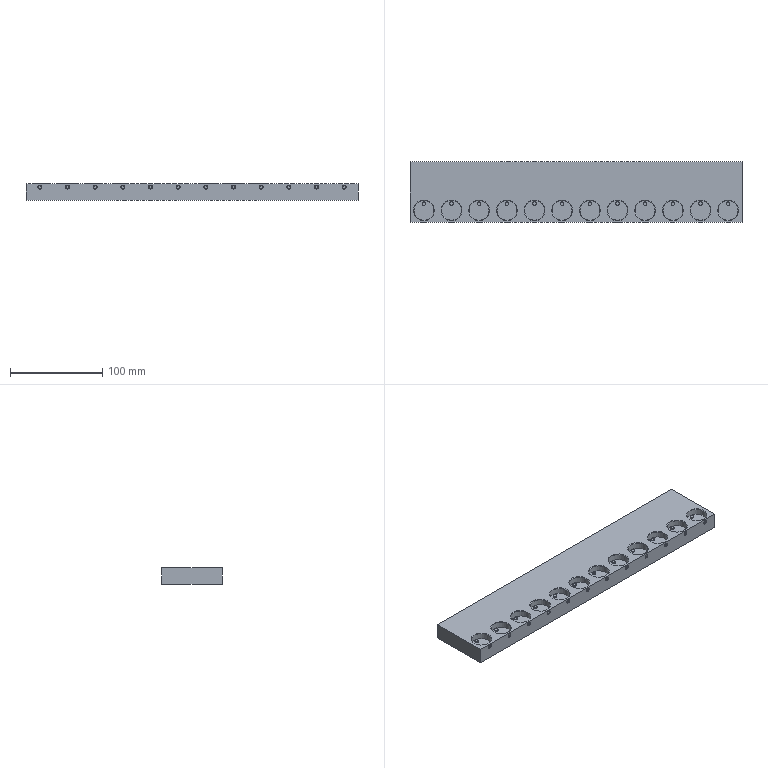NC program | NX | posted with a generic post | part box 360 x 66 x 17.6 mm
Lines 1 to 734 of 61781:
N10 G17 G21 G94 G90
(1 , TOOL : D4-T1)
N12 T01 M6
N14 G54
N16 G17 G0 G90 X-16.694 Y-15.384 B0. C0. S8000 M3
N18 G43 Z103. H1
N20 G94 G1 Z3. F5000.
N22 G3 X-16.694 Y-15.384 Z2.941 I1.694 J0.608 F2000.
N24 X-16.694 Y-15.384 Z2.882 I1.694 J0.608
N26 X-16.694 Y-15.384 Z2.822 I1.694 J0.608
N28 X-16.694 Y-15.384 Z2.763 I1.694 J0.608
N30 X-16.694 Y-15.384 Z2.704 I1.694 J0.608
N32 X-16.694 Y-15.384 Z2.645 I1.694 J0.608
N34 X-16.694 Y-15.384 Z2.585 I1.694 J0.608
N36 X-16.694 Y-15.384 Z2.526 I1.694 J0.608
N38 X-16.694 Y-15.384 Z2.467 I1.694 J0.608
N40 X-16.694 Y-15.384 Z2.408 I1.694 J0.608
N42 X-16.694 Y-15.384 Z2.349 I1.694 J0.608
N44 X-16.694 Y-15.384 Z2.289 I1.694 J0.608
N46 X-16.694 Y-15.384 Z2.23 I1.694 J0.608
N48 X-16.694 Y-15.384 Z2.171 I1.694 J0.608
N50 X-16.694 Y-15.384 Z2.112 I1.694 J0.608
N52 X-16.694 Y-15.384 Z2.053 I1.694 J0.608
N54 X-16.694 Y-15.384 Z1.993 I1.694 J0.608
N56 X-16.694 Y-15.384 Z1.934 I1.694 J0.608
N58 X-16.694 Y-15.384 Z1.875 I1.694 J0.608
N60 X-16.694 Y-15.384 Z1.816 I1.694 J0.608
N62 X-16.694 Y-15.384 Z1.756 I1.694 J0.608
N64 X-16.694 Y-15.384 Z1.697 I1.694 J0.608
N66 X-16.694 Y-15.384 Z1.638 I1.694 J0.608
N68 X-16.694 Y-15.384 Z1.579 I1.694 J0.608
N70 X-16.694 Y-15.384 Z1.52 I1.694 J0.608
N72 X-16.694 Y-15.384 Z1.46 I1.694 J0.608
N74 X-16.694 Y-15.384 Z1.401 I1.694 J0.608
N76 X-16.694 Y-15.384 Z1.342 I1.694 J0.608
N78 X-16.694 Y-15.384 Z1.283 I1.694 J0.608
N80 X-16.694 Y-15.384 Z1.223 I1.694 J0.608
N82 X-16.694 Y-15.384 Z1.164 I1.694 J0.608
N84 X-16.694 Y-15.384 Z1.105 I1.694 J0.608
N86 X-16.694 Y-15.384 Z1.046 I1.694 J0.608
N88 X-16.694 Y-15.384 Z0.987 I1.694 J0.608
N90 X-16.694 Y-15.384 Z0.927 I1.694 J0.608
N92 X-16.694 Y-15.384 Z0.868 I1.694 J0.608
N94 X-16.694 Y-15.384 Z0.809 I1.694 J0.608
N96 X-16.694 Y-15.384 Z0.75 I1.694 J0.608
N98 X-16.694 Y-15.384 Z0.69 I1.694 J0.608
N100 X-16.694 Y-15.384 Z0.631 I1.694 J0.608
N102 X-16.694 Y-15.384 Z0.572 I1.694 J0.608
N104 X-16.694 Y-15.384 Z0.513 I1.694 J0.608
N106 X-16.694 Y-15.384 Z0.454 I1.694 J0.608
N108 X-16.694 Y-15.384 Z0.394 I1.694 J0.608
N110 X-16.694 Y-15.384 Z0.335 I1.694 J0.608
N112 X-16.694 Y-15.384 Z0.276 I1.694 J0.608
N114 X-16.694 Y-15.384 Z0.217 I1.694 J0.608
N116 X-16.694 Y-15.384 Z0.158 I1.694 J0.608
N118 X-16.694 Y-15.384 Z0.098 I1.694 J0.608
N120 X-15. Y-12.976 Z0.057 R-1.8
N122 G1 Y-13.034
N124 Y-12.976
N126 Y-11.176
N128 G3 X-16.824 Y-13. R1.824
N130 X-15. Y-11.176 R-1.824
N132 G1 Y-8.776
N134 G3 X-19.224 Y-13. R4.224
N136 X-15. Y-8.776 R-4.224
N138 G1 Y-6.376
N140 G3 X-21.624 Y-13. R6.624
N142 X-15. Y-6.376 R-6.624
N144 G1 Y-3.976
N146 G3 X-24.024 Y-13. R9.024
N148 X-15. Y-3.976 R-9.024
N150 G1 Y-5.976
N152 G0 Z6.
N154 X-13.237 Y-13.804
N156 G1 Z0.057 F5000.
N158 G3 X-13.237 Y-13.804 Z-0.002 I-1.763 J0.365 F2000.
N160 X-13.237 Y-13.804 Z-0.061 I-1.763 J0.365
N162 X-13.237 Y-13.804 Z-0.121 I-1.763 J0.365
N164 X-13.237 Y-13.804 Z-0.18 I-1.763 J0.365
N166 X-13.237 Y-13.804 Z-0.239 I-1.763 J0.365
N168 X-13.237 Y-13.804 Z-0.298 I-1.763 J0.365
N170 X-13.237 Y-13.804 Z-0.357 I-1.763 J0.365
N172 X-13.237 Y-13.804 Z-0.417 I-1.763 J0.365
N174 X-15. Y-11.639 Z-0.433 R1.8
N176 X-16.361 Y-13. R1.361
N178 X-15. Y-11.639 R-1.361
N180 G1 Y-9.239
N182 G3 X-18.761 Y-13. R3.761
N184 X-15. Y-9.239 R-3.761
N186 G1 Y-6.839
N188 G3 X-21.161 Y-13. R6.161
N190 X-15. Y-6.839 R-6.161
N192 G1 Y-4.439
N194 G3 X-23.561 Y-13. R8.561
N196 X-15. Y-4.439 R-8.561
N198 G1 Y-6.439
N200 G0 Z3.057
N202 X-13.237 Y-13.815
N204 G1 Z-0.433 F5000.
N206 G3 X-13.237 Y-13.815 Z-0.493 I-1.763 J0.365 F2000.
N208 X-13.237 Y-13.815 Z-0.552 I-1.763 J0.365
N210 X-13.237 Y-13.815 Z-0.611 I-1.763 J0.365
N212 X-13.237 Y-13.815 Z-0.67 I-1.763 J0.365
N214 X-13.237 Y-13.815 Z-0.729 I-1.763 J0.365
N216 X-13.237 Y-13.815 Z-0.789 I-1.763 J0.365
N218 X-13.237 Y-13.815 Z-0.848 I-1.763 J0.365
N220 X-13.237 Y-13.815 Z-0.907 I-1.763 J0.365
N222 X-15. Y-11.65 Z-0.924 R1.8
N224 X-16.35 Y-13. R1.35
N226 X-15. Y-11.65 R-1.35
N228 G1 Y-9.25
N230 G3 X-18.75 Y-13. R3.75
N232 X-15. Y-9.25 R-3.75
N234 G1 Y-6.85
N236 G3 X-21.15 Y-13. R6.15
N238 X-15. Y-6.85 R-6.15
N240 G1 Y-4.45
N242 G3 X-23.55 Y-13. R8.55
N244 X-15. Y-4.45 R-8.55
N246 G1 Y-6.45
N248 G0 Z2.567
N250 X-13.237 Y-13.815
N252 G1 Z-0.924 F5000.
N254 G3 X-13.237 Y-13.815 Z-0.983 I-1.763 J0.365 F2000.
N256 X-13.237 Y-13.815 Z-1.042 I-1.763 J0.365
N258 X-13.237 Y-13.815 Z-1.101 I-1.763 J0.365
N260 X-13.237 Y-13.815 Z-1.161 I-1.763 J0.365
N262 X-13.237 Y-13.815 Z-1.22 I-1.763 J0.365
N264 X-13.237 Y-13.815 Z-1.279 I-1.763 J0.365
N266 X-13.237 Y-13.815 Z-1.338 I-1.763 J0.365
N268 X-13.237 Y-13.815 Z-1.398 I-1.763 J0.365
N270 X-15. Y-11.65 Z-1.414 R1.8
N272 X-16.35 Y-13. R1.35
N274 X-15. Y-11.65 R-1.35
N276 G1 Y-9.25
N278 G3 X-18.75 Y-13. R3.75
N280 X-15. Y-9.25 R-3.75
N282 G1 Y-6.85
N284 G3 X-21.15 Y-13. R6.15
N286 X-15. Y-6.85 R-6.15
N288 G1 Y-4.45
N290 G3 X-23.55 Y-13. R8.55
N292 X-15. Y-4.45 R-8.55
N294 G1 Y-6.45
N296 G0 Z2.076
N298 X-13.237 Y-13.815
N300 G1 Z-1.414 F5000.
N302 G3 X-13.237 Y-13.815 Z-1.474 I-1.763 J0.365 F2000.
N304 X-13.237 Y-13.815 Z-1.533 I-1.763 J0.365
N306 X-13.237 Y-13.815 Z-1.592 I-1.763 J0.365
N308 X-13.237 Y-13.815 Z-1.651 I-1.763 J0.365
N310 X-13.237 Y-13.815 Z-1.71 I-1.763 J0.365
N312 X-13.237 Y-13.815 Z-1.77 I-1.763 J0.365
N314 X-13.237 Y-13.815 Z-1.829 I-1.763 J0.365
N316 X-13.237 Y-13.815 Z-1.888 I-1.763 J0.365
N318 X-15. Y-11.65 Z-1.905 R1.8
N320 X-16.35 Y-13. R1.35
N322 X-15. Y-11.65 R-1.35
N324 G1 Y-9.25
N326 G3 X-18.75 Y-13. R3.75
N328 X-15. Y-9.25 R-3.75
N330 G1 Y-6.85
N332 G3 X-21.15 Y-13. R6.15
N334 X-15. Y-6.85 R-6.15
N336 G1 Y-4.45
N338 G3 X-23.55 Y-13. R8.55
N340 X-15. Y-4.45 R-8.55
N342 G1 Y-6.45
N344 G0 Z1.586
N346 X-13.237 Y-13.815
N348 G1 Z-1.905 F5000.
N350 G3 X-13.237 Y-13.815 Z-1.964 I-1.763 J0.365 F2000.
N352 X-13.237 Y-13.815 Z-2.023 I-1.763 J0.365
N354 X-13.237 Y-13.815 Z-2.082 I-1.763 J0.365
N356 X-13.237 Y-13.815 Z-2.142 I-1.763 J0.365
N358 X-13.237 Y-13.815 Z-2.201 I-1.763 J0.365
N360 X-13.237 Y-13.815 Z-2.26 I-1.763 J0.365
N362 X-13.237 Y-13.815 Z-2.319 I-1.763 J0.365
N364 X-13.237 Y-13.815 Z-2.379 I-1.763 J0.365
N366 X-15. Y-11.65 Z-2.395 R1.8
N368 X-16.35 Y-13. R1.35
N370 X-15. Y-11.65 R-1.35
N372 G1 Y-9.25
N374 G3 X-18.75 Y-13. R3.75
N376 X-15. Y-9.25 R-3.75
N378 G1 Y-6.85
N380 G3 X-21.15 Y-13. R6.15
N382 X-15. Y-6.85 R-6.15
N384 G1 Y-4.45
N386 G3 X-23.55 Y-13. R8.55
N388 X-15. Y-4.45 R-8.55
N390 G1 Y-6.45
N392 G0 Z1.095
N394 X-13.237 Y-13.815
N396 G1 Z-2.395 F5000.
N398 G3 X-13.237 Y-13.815 Z-2.454 I-1.763 J0.365 F2000.
N400 X-13.237 Y-13.815 Z-2.514 I-1.763 J0.365
N402 X-13.237 Y-13.815 Z-2.573 I-1.763 J0.365
N404 X-13.237 Y-13.815 Z-2.632 I-1.763 J0.365
N406 X-13.237 Y-13.815 Z-2.691 I-1.763 J0.365
N408 X-13.237 Y-13.815 Z-2.751 I-1.763 J0.365
N410 X-13.237 Y-13.815 Z-2.81 I-1.763 J0.365
N412 X-13.237 Y-13.815 Z-2.869 I-1.763 J0.365
N414 X-15. Y-11.65 Z-2.886 R1.8
N416 X-16.35 Y-13. R1.35
N418 X-15. Y-11.65 R-1.35
N420 G1 Y-9.25
N422 G3 X-18.75 Y-13. R3.75
N424 X-15. Y-9.25 R-3.75
N426 G1 Y-6.85
N428 G3 X-21.15 Y-13. R6.15
N430 X-15. Y-6.85 R-6.15
N432 G1 Y-4.45
N434 G3 X-23.55 Y-13. R8.55
N436 X-15. Y-4.45 R-8.55
N438 G1 Y-6.45
N440 G0 Z0.605
N442 X-13.237 Y-13.815
N444 G1 Z-2.886 F5000.
N446 G3 X-13.237 Y-13.815 Z-2.945 I-1.763 J0.365 F2000.
N448 X-13.237 Y-13.815 Z-3.004 I-1.763 J0.365
N450 X-13.237 Y-13.815 Z-3.063 I-1.763 J0.365
N452 X-13.237 Y-13.815 Z-3.123 I-1.763 J0.365
N454 X-13.237 Y-13.815 Z-3.182 I-1.763 J0.365
N456 X-13.237 Y-13.815 Z-3.241 I-1.763 J0.365
N458 X-13.237 Y-13.815 Z-3.3 I-1.763 J0.365
N460 X-13.237 Y-13.815 Z-3.359 I-1.763 J0.365
N462 X-15. Y-11.65 Z-3.376 R1.8
N464 X-16.35 Y-13. R1.35
N466 X-15. Y-11.65 R-1.35
N468 G1 Y-9.25
N470 G3 X-18.75 Y-13. R3.75
N472 X-15. Y-9.25 R-3.75
N474 G1 Y-6.85
N476 G3 X-21.15 Y-13. R6.15
N478 X-15. Y-6.85 R-6.15
N480 G1 Y-4.45
N482 G3 X-23.55 Y-13. R8.55
N484 X-15. Y-4.45 R-8.55
N486 G1 Y-6.45
N488 G0 Z0.114
N490 X-13.237 Y-13.815
N492 G1 Z-3.376 F5000.
N494 G3 X-13.237 Y-13.815 Z-3.435 I-1.763 J0.365 F2000.
N496 X-13.237 Y-13.815 Z-3.495 I-1.763 J0.365
N498 X-13.237 Y-13.815 Z-3.554 I-1.763 J0.365
N500 X-13.237 Y-13.815 Z-3.613 I-1.763 J0.365
N502 X-13.237 Y-13.815 Z-3.672 I-1.763 J0.365
N504 X-13.237 Y-13.815 Z-3.732 I-1.763 J0.365
N506 X-13.237 Y-13.815 Z-3.791 I-1.763 J0.365
N508 X-13.237 Y-13.815 Z-3.85 I-1.763 J0.365
N510 X-15. Y-11.65 Z-3.867 R1.8
N512 X-16.35 Y-13. R1.35
N514 X-15. Y-11.65 R-1.35
N516 G1 Y-9.25
N518 G3 X-18.75 Y-13. R3.75
N520 X-15. Y-9.25 R-3.75
N522 G1 Y-6.85
N524 G3 X-21.15 Y-13. R6.15
N526 X-15. Y-6.85 R-6.15
N528 G1 Y-4.45
N530 G3 X-23.55 Y-13. R8.55
N532 X-15. Y-4.45 R-8.55
N534 G1 Y-6.45
N536 G0 Z-0.376
N538 X-13.237 Y-13.815
N540 G1 Z-3.867 F5000.
N542 G3 X-13.237 Y-13.815 Z-3.926 I-1.763 J0.365 F2000.
N544 X-13.237 Y-13.815 Z-3.985 I-1.763 J0.365
N546 X-13.237 Y-13.815 Z-4.044 I-1.763 J0.365
N548 X-13.237 Y-13.815 Z-4.104 I-1.763 J0.365
N550 X-13.237 Y-13.815 Z-4.163 I-1.763 J0.365
N552 X-13.237 Y-13.815 Z-4.222 I-1.763 J0.365
N554 X-13.237 Y-13.815 Z-4.281 I-1.763 J0.365
N556 X-13.237 Y-13.815 Z-4.34 I-1.763 J0.365
N558 X-15. Y-11.65 Z-4.357 R1.8
N560 X-16.35 Y-13. R1.35
N562 X-15. Y-11.65 R-1.35
N564 G1 Y-9.25
N566 G3 X-18.75 Y-13. R3.75
N568 X-15. Y-9.25 R-3.75
N570 G1 Y-6.85
N572 G3 X-21.15 Y-13. R6.15
N574 X-15. Y-6.85 R-6.15
N576 G1 Y-4.45
N578 G3 X-23.55 Y-13. R8.55
N580 X-15. Y-4.45 R-8.55
N582 G1 Y-6.45
N584 G0 Z-0.867
N586 X-13.237 Y-13.815
N588 G1 Z-4.357 F5000.
N590 G3 X-13.237 Y-13.815 Z-4.416 I-1.763 J0.365 F2000.
N592 X-13.237 Y-13.815 Z-4.476 I-1.763 J0.365
N594 X-13.237 Y-13.815 Z-4.535 I-1.763 J0.365
N596 X-13.237 Y-13.815 Z-4.594 I-1.763 J0.365
N598 X-13.237 Y-13.815 Z-4.653 I-1.763 J0.365
N600 X-13.237 Y-13.815 Z-4.712 I-1.763 J0.365
N602 X-13.237 Y-13.815 Z-4.772 I-1.763 J0.365
N604 X-13.237 Y-13.815 Z-4.831 I-1.763 J0.365
N606 X-15. Y-11.65 Z-4.848 R1.8
N608 X-16.35 Y-13. R1.35
N610 X-15. Y-11.65 R-1.35
N612 G1 Y-9.25
N614 G3 X-18.75 Y-13. R3.75
N616 X-15. Y-9.25 R-3.75
N618 G1 Y-6.85
N620 G3 X-21.15 Y-13. R6.15
N622 X-15. Y-6.85 R-6.15
N624 G1 Y-4.45
N626 G3 X-23.55 Y-13. R8.55
N628 X-15. Y-4.45 R-8.55
N630 G1 Y-6.45
N632 G0 Z-1.357
N634 X-13.237 Y-13.815
N636 G1 Z-4.848 F5000.
N638 G3 X-13.237 Y-13.815 Z-4.907 I-1.763 J0.365 F2000.
N640 X-13.237 Y-13.815 Z-4.966 I-1.763 J0.365
N642 X-13.237 Y-13.815 Z-5.025 I-1.763 J0.365
N644 X-13.237 Y-13.815 Z-5.084 I-1.763 J0.365
N646 X-13.237 Y-13.815 Z-5.144 I-1.763 J0.365
N648 X-13.237 Y-13.815 Z-5.203 I-1.763 J0.365
N650 X-13.237 Y-13.815 Z-5.262 I-1.763 J0.365
N652 X-13.237 Y-13.815 Z-5.321 I-1.763 J0.365
N654 X-15. Y-11.65 Z-5.338 R1.8
N656 X-16.35 Y-13. R1.35
N658 X-15. Y-11.65 R-1.35
N660 G1 Y-9.25
N662 G3 X-18.75 Y-13. R3.75
N664 X-15. Y-9.25 R-3.75
N666 G1 Y-6.85
N668 G3 X-21.15 Y-13. R6.15
N670 X-15. Y-6.85 R-6.15
N672 G1 Y-4.45
N674 G3 X-23.55 Y-13. R8.55
N676 X-15. Y-4.45 R-8.55
N678 G1 Y-6.45
N680 G0 Z-1.848
N682 X-12.353 Y-9.607
N684 G1 Z-5.338 F5000.
N686 G3 X-12.353 Y-9.607 Z-5.397 I1.48 J-1.025 F2000.
N688 X-12.353 Y-9.607 Z-5.457 I1.48 J-1.025
N690 X-12.353 Y-9.607 Z-5.516 I1.48 J-1.025
N692 X-12.353 Y-9.607 Z-5.575 I1.48 J-1.025
N694 X-12.353 Y-9.607 Z-5.634 I1.48 J-1.025
N696 X-12.353 Y-9.607 Z-5.693 I1.48 J-1.025
N698 X-12.353 Y-9.607 Z-5.753 I1.48 J-1.025
N700 X-12.353 Y-9.607 Z-5.812 I1.48 J-1.025
N702 X-11.577 Y-12.289 Z-5.829 R1.8
N704 G2 X-11.296 Y-12.414 R8.758
N706 G3 X-18.704 Y-12.414 R3.75
N708 G2 X-11.577 Y-12.289 R8.758
N710 G1 X-12.515 Y-14.498
N712 G2 X-9.942 Y-16.498 R6.358
N714 G3 X-20.058 Y-16.498 R-6.15
N716 G2 X-12.515 Y-14.498 R6.358
N718 G1 X-13.453 Y-16.707
N720 G2 X-11.049 Y-20.582 R3.958
N722 G3 X-18.951 Y-20.582 R-8.55
N724 G2 X-13.453 Y-16.707 R3.958
N726 G1 X-12.671 Y-14.866
N728 G0 Z-2.338
N730 X-13.237 Y-11.415
N732 G1 Z-5.829 F5000.
N734 G3 X-13.237 Y-11.415 Z-5.888 I-1.763 J0.365 F2000.
N736 X-13.237 Y-11.415 Z-5.947 I-1.763 J0.365
N738 X-13.237 Y-11.415 Z-6.006 I-1.763 J0.365
N740 X-13.237 Y-11.415 Z-6.065 I-1.763 J0.365
N742 X-13.237 Y-11.415 Z-6.125 I-1.763 J0.365
N744 X-13.237 Y-11.415 Z-6.184 I-1.763 J0.365
N746 X-13.237 Y-11.415 Z-6.243 I-1.763 J0.365
N748 X-13.237 Y-11.415 Z-6.302 I-1.763 J0.365
N750 X-15. Y-9.25 Z-6.319 R1.8
N752 X-18.658 Y-12.176 R3.75
N754 G2 X-11.342 Y-12.176 R8.955
N756 G3 X-15. Y-9.25 R3.75
N758 G1 Y-6.85
N760 G3 X-20.174 Y-16.325 R6.15
N762 G2 X-9.826 Y-16.325 R6.555
N764 G3 X-15. Y-6.85 R6.15
N766 G1 Y-4.45
N768 G3 X-19.153 Y-20.474 R8.55
N770 G2 X-10.847 Y-20.474 R-4.155
N772 G3 X-15. Y-4.45 R8.55
N774 G1 Y-6.45
N776 G0 Z103.
(1_COPY , TOOL : D4-T1)
N778 X-46.694 Y-15.384
N780 G1 Z3. F5000.
N782 G3 X-46.694 Y-15.384 Z2.941 I1.694 J0.608 F2000.
N784 X-46.694 Y-15.384 Z2.882 I1.694 J0.608
N786 X-46.694 Y-15.384 Z2.822 I1.694 J0.608
N788 X-46.694 Y-15.384 Z2.763 I1.694 J0.608
N790 X-46.694 Y-15.384 Z2.704 I1.694 J0.608
N792 X-46.694 Y-15.384 Z2.645 I1.694 J0.608
N794 X-46.694 Y-15.384 Z2.585 I1.694 J0.608
N796 X-46.694 Y-15.384 Z2.526 I1.694 J0.608
N798 X-46.694 Y-15.384 Z2.467 I1.694 J0.608
N800 X-46.694 Y-15.384 Z2.408 I1.694 J0.608
N802 X-46.694 Y-15.384 Z2.349 I1.694 J0.608
N804 X-46.694 Y-15.384 Z2.289 I1.694 J0.608
N806 X-46.694 Y-15.384 Z2.23 I1.694 J0.608
N808 X-46.694 Y-15.384 Z2.171 I1.694 J0.608
N810 X-46.694 Y-15.384 Z2.112 I1.694 J0.608
N812 X-46.694 Y-15.384 Z2.053 I1.694 J0.608
N814 X-46.694 Y-15.384 Z1.993 I1.694 J0.608
N816 X-46.694 Y-15.384 Z1.934 I1.694 J0.608
N818 X-46.694 Y-15.384 Z1.875 I1.694 J0.608
N820 X-46.694 Y-15.384 Z1.816 I1.694 J0.608
N822 X-46.694 Y-15.384 Z1.756 I1.694 J0.608
N824 X-46.694 Y-15.384 Z1.697 I1.694 J0.608
N826 X-46.694 Y-15.384 Z1.638 I1.694 J0.608
N828 X-46.694 Y-15.384 Z1.579 I1.694 J0.608
N830 X-46.694 Y-15.384 Z1.52 I1.694 J0.608
N832 X-46.694 Y-15.384 Z1.46 I1.694 J0.608
N834 X-46.694 Y-15.384 Z1.401 I1.694 J0.608
N836 X-46.694 Y-15.384 Z1.342 I1.694 J0.608
N838 X-46.694 Y-15.384 Z1.283 I1.694 J0.608
N840 X-46.694 Y-15.384 Z1.223 I1.694 J0.608
N842 X-46.694 Y-15.384 Z1.164 I1.694 J0.608
N844 X-46.694 Y-15.384 Z1.105 I1.694 J0.608
N846 X-46.694 Y-15.384 Z1.046 I1.694 J0.608
N848 X-46.694 Y-15.384 Z0.987 I1.694 J0.608
N850 X-46.694 Y-15.384 Z0.927 I1.694 J0.608
N852 X-46.694 Y-15.384 Z0.868 I1.694 J0.608
N854 X-46.694 Y-15.384 Z0.809 I1.694 J0.608
N856 X-46.694 Y-15.384 Z0.75 I1.694 J0.608
N858 X-46.694 Y-15.384 Z0.69 I1.694 J0.608
N860 X-46.694 Y-15.384 Z0.631 I1.694 J0.608
N862 X-46.694 Y-15.384 Z0.572 I1.694 J0.608
N864 X-46.694 Y-15.384 Z0.513 I1.694 J0.608
N866 X-46.694 Y-15.384 Z0.454 I1.694 J0.608
N868 X-46.694 Y-15.384 Z0.394 I1.694 J0.608
N870 X-46.694 Y-15.384 Z0.335 I1.694 J0.608
N872 X-46.694 Y-15.384 Z0.276 I1.694 J0.608
N874 X-46.694 Y-15.384 Z0.217 I1.694 J0.608
N876 X-46.694 Y-15.384 Z0.158 I1.694 J0.608
N878 X-46.694 Y-15.384 Z0.098 I1.694 J0.608
N880 X-45. Y-12.976 Z0.057 R-1.8
N882 G1 Y-13.034
N884 Y-12.976
N886 Y-11.176
N888 G3 X-46.824 Y-13. R1.824
N890 X-45. Y-11.176 R-1.824
N892 G1 Y-8.776
N894 G3 X-49.224 Y-13. R4.224
N896 X-45. Y-8.776 R-4.224
N898 G1 Y-6.376
N900 G3 X-51.624 Y-13. R6.624
N902 X-45. Y-6.376 R-6.624
N904 G1 Y-3.976
N906 G3 X-54.024 Y-13. R9.024
N908 X-45. Y-3.976 R-9.024
N910 G1 Y-5.976
N912 G0 Z6.
N914 X-43.237 Y-13.804
N916 G1 Z0.057 F5000.
N918 G3 X-43.237 Y-13.804 Z-0.002 I-1.763 J0.365 F2000.
N920 X-43.237 Y-13.804 Z-0.061 I-1.763 J0.365
N922 X-43.237 Y-13.804 Z-0.121 I-1.763 J0.365
N924 X-43.237 Y-13.804 Z-0.18 I-1.763 J0.365
N926 X-43.237 Y-13.804 Z-0.239 I-1.763 J0.365
N928 X-43.237 Y-13.804 Z-0.298 I-1.763 J0.365
N930 X-43.237 Y-13.804 Z-0.357 I-1.763 J0.365
N932 X-43.237 Y-13.804 Z-0.417 I-1.763 J0.365
N934 X-45. Y-11.639 Z-0.433 R1.8
N936 X-46.361 Y-13. R1.361
N938 X-45. Y-11.639 R-1.361
N940 G1 Y-9.239
N942 G3 X-48.761 Y-13. R3.761
N944 X-45. Y-9.239 R-3.761
N946 G1 Y-6.839
N948 G3 X-51.161 Y-13. R6.161
N950 X-45. Y-6.839 R-6.161
N952 G1 Y-4.439
N954 G3 X-53.561 Y-13. R8.561
N956 X-45. Y-4.439 R-8.561
N958 G1 Y-6.439
N960 G0 Z3.057
N962 X-43.237 Y-13.815
N964 G1 Z-0.433 F5000.
N966 G3 X-43.237 Y-13.815 Z-0.493 I-1.763 J0.365 F2000.
N968 X-43.237 Y-13.815 Z-0.552 I-1.763 J0.365
N970 X-43.237 Y-13.815 Z-0.611 I-1.763 J0.365
N972 X-43.237 Y-13.815 Z-0.67 I-1.763 J0.365
N974 X-43.237 Y-13.815 Z-0.729 I-1.763 J0.365
N976 X-43.237 Y-13.815 Z-0.789 I-1.763 J0.365
N978 X-43.237 Y-13.815 Z-0.848 I-1.763 J0.365
N980 X-43.237 Y-13.815 Z-0.907 I-1.763 J0.365
N982 X-45. Y-11.65 Z-0.924 R1.8
N984 X-46.35 Y-13. R1.35
N986 X-45. Y-11.65 R-1.35
N988 G1 Y-9.25
N990 G3 X-48.75 Y-13. R3.75
N992 X-45. Y-9.25 R-3.75
N994 G1 Y-6.85
N996 G3 X-51.15 Y-13. R6.15
N998 X-45. Y-6.85 R-6.15
N1000 G1 Y-4.45
N1002 G3 X-53.55 Y-13. R8.55
N1004 X-45. Y-4.45 R-8.55
N1006 G1 Y-6.45
N1008 G0 Z2.567
N1010 X-43.237 Y-13.815
N1012 G1 Z-0.924 F5000.
N1014 G3 X-43.237 Y-13.815 Z-0.983 I-1.763 J0.365 F2000.
N1016 X-43.237 Y-13.815 Z-1.042 I-1.763 J0.365
N1018 X-43.237 Y-13.815 Z-1.101 I-1.763 J0.365
N1020 X-43.237 Y-13.815 Z-1.161 I-1.763 J0.365
N1022 X-43.237 Y-13.815 Z-1.22 I-1.763 J0.365
N1024 X-43.237 Y-13.815 Z-1.279 I-1.763 J0.365
N1026 X-43.237 Y-13.815 Z-1.338 I-1.763 J0.365
N1028 X-43.237 Y-13.815 Z-1.398 I-1.763 J0.365
N1030 X-45. Y-11.65 Z-1.414 R1.8
N1032 X-46.35 Y-13. R1.35
N1034 X-45. Y-11.65 R-1.35
N1036 G1 Y-9.25
N1038 G3 X-48.75 Y-13. R3.75
N1040 X-45. Y-9.25 R-3.75
N1042 G1 Y-6.85
N1044 G3 X-51.15 Y-13. R6.15
N1046 X-45. Y-6.85 R-6.15
N1048 G1 Y-4.45
N1050 G3 X-53.55 Y-13. R8.55
N1052 X-45. Y-4.45 R-8.55
N1054 G1 Y-6.45
N1056 G0 Z2.076
N1058 X-43.237 Y-13.815
N1060 G1 Z-1.414 F5000.
N1062 G3 X-43.237 Y-13.815 Z-1.474 I-1.763 J0.365 F2000.
N1064 X-43.237 Y-13.815 Z-1.533 I-1.763 J0.365
N1066 X-43.237 Y-13.815 Z-1.592 I-1.763 J0.365
N1068 X-43.237 Y-13.815 Z-1.651 I-1.763 J0.365
N1070 X-43.237 Y-13.815 Z-1.71 I-1.763 J0.365
N1072 X-43.237 Y-13.815 Z-1.77 I-1.763 J0.365
N1074 X-43.237 Y-13.815 Z-1.829 I-1.763 J0.365
N1076 X-43.237 Y-13.815 Z-1.888 I-1.763 J0.365
N1078 X-45. Y-11.65 Z-1.905 R1.8
N1080 X-46.35 Y-13. R1.35
N1082 X-45. Y-11.65 R-1.35
N1084 G1 Y-9.25
N1086 G3 X-48.75 Y-13. R3.75
N1088 X-45. Y-9.25 R-3.75
N1090 G1 Y-6.85
N1092 G3 X-51.15 Y-13. R6.15
N1094 X-45. Y-6.85 R-6.15
N1096 G1 Y-4.45
N1098 G3 X-53.55 Y-13. R8.55
N1100 X-45. Y-4.45 R-8.55
N1102 G1 Y-6.45
N1104 G0 Z1.586
N1106 X-43.237 Y-13.815
N1108 G1 Z-1.905 F5000.
N1110 G3 X-43.237 Y-13.815 Z-1.964 I-1.763 J0.365 F2000.
N1112 X-43.237 Y-13.815 Z-2.023 I-1.763 J0.365
N1114 X-43.237 Y-13.815 Z-2.082 I-1.763 J0.365
N1116 X-43.237 Y-13.815 Z-2.142 I-1.763 J0.365
N1118 X-43.237 Y-13.815 Z-2.201 I-1.763 J0.365
N1120 X-43.237 Y-13.815 Z-2.26 I-1.763 J0.365
N1122 X-43.237 Y-13.815 Z-2.319 I-1.763 J0.365
N1124 X-43.237 Y-13.815 Z-2.379 I-1.763 J0.365
N1126 X-45. Y-11.65 Z-2.395 R1.8
N1128 X-46.35 Y-13. R1.35
N1130 X-45. Y-11.65 R-1.35
N1132 G1 Y-9.25
N1134 G3 X-48.75 Y-13. R3.75
N1136 X-45. Y-9.25 R-3.75
N1138 G1 Y-6.85
N1140 G3 X-51.15 Y-13. R6.15
N1142 X-45. Y-6.85 R-6.15
N1144 G1 Y-4.45
N1146 G3 X-53.55 Y-13. R8.55
N1148 X-45. Y-4.45 R-8.55
N1150 G1 Y-6.45
N1152 G0 Z1.095
N1154 X-43.237 Y-13.815
N1156 G1 Z-2.395 F5000.
N1158 G3 X-43.237 Y-13.815 Z-2.454 I-1.763 J0.365 F2000.
N1160 X-43.237 Y-13.815 Z-2.514 I-1.763 J0.365
N1162 X-43.237 Y-13.815 Z-2.573 I-1.763 J0.365
N1164 X-43.237 Y-13.815 Z-2.632 I-1.763 J0.365
N1166 X-43.237 Y-13.815 Z-2.691 I-1.763 J0.365
N1168 X-43.237 Y-13.815 Z-2.751 I-1.763 J0.365
N1170 X-43.237 Y-13.815 Z-2.81 I-1.763 J0.365
N1172 X-43.237 Y-13.815 Z-2.869 I-1.763 J0.365
N1174 X-45. Y-11.65 Z-2.886 R1.8
N1176 X-46.35 Y-13. R1.35
N1178 X-45. Y-11.65 R-1.35
N1180 G1 Y-9.25
N1182 G3 X-48.75 Y-13. R3.75
N1184 X-45. Y-9.25 R-3.75
N1186 G1 Y-6.85
N1188 G3 X-51.15 Y-13. R6.15
N1190 X-45. Y-6.85 R-6.15
N1192 G1 Y-4.45
N1194 G3 X-53.55 Y-13. R8.55
N1196 X-45. Y-4.45 R-8.55
N1198 G1 Y-6.45
N1200 G0 Z0.605
N1202 X-43.237 Y-13.815
N1204 G1 Z-2.886 F5000.
N1206 G3 X-43.237 Y-13.815 Z-2.945 I-1.763 J0.365 F2000.
N1208 X-43.237 Y-13.815 Z-3.004 I-1.763 J0.365
N1210 X-43.237 Y-13.815 Z-3.063 I-1.763 J0.365
N1212 X-43.237 Y-13.815 Z-3.123 I-1.763 J0.365
N1214 X-43.237 Y-13.815 Z-3.182 I-1.763 J0.365
N1216 X-43.237 Y-13.815 Z-3.241 I-1.763 J0.365
N1218 X-43.237 Y-13.815 Z-3.3 I-1.763 J0.365
N1220 X-43.237 Y-13.815 Z-3.359 I-1.763 J0.365
N1222 X-45. Y-11.65 Z-3.376 R1.8
N1224 X-46.35 Y-13. R1.35
N1226 X-45. Y-11.65 R-1.35
N1228 G1 Y-9.25
N1230 G3 X-48.75 Y-13. R3.75
N1232 X-45. Y-9.25 R-3.75
N1234 G1 Y-6.85
N1236 G3 X-51.15 Y-13. R6.15
N1238 X-45. Y-6.85 R-6.15
N1240 G1 Y-4.45
N1242 G3 X-53.55 Y-13. R8.55
N1244 X-45. Y-4.45 R-8.55
N1246 G1 Y-6.45
N1248 G0 Z0.114
N1250 X-43.237 Y-13.815
N1252 G1 Z-3.376 F5000.
N1254 G3 X-43.237 Y-13.815 Z-3.435 I-1.763 J0.365 F2000.
N1256 X-43.237 Y-13.815 Z-3.495 I-1.763 J0.365
N1258 X-43.237 Y-13.815 Z-3.554 I-1.763 J0.365
N1260 X-43.237 Y-13.815 Z-3.613 I-1.763 J0.365
N1262 X-43.237 Y-13.815 Z-3.672 I-1.763 J0.365
N1264 X-43.237 Y-13.815 Z-3.732 I-1.763 J0.365
N1266 X-43.237 Y-13.815 Z-3.791 I-1.763 J0.365
N1268 X-43.237 Y-13.815 Z-3.85 I-1.763 J0.365
N1270 X-45. Y-11.65 Z-3.867 R1.8
N1272 X-46.35 Y-13. R1.35
N1274 X-45. Y-11.65 R-1.35
N1276 G1 Y-9.25
N1278 G3 X-48.75 Y-13. R3.75
N1280 X-45. Y-9.25 R-3.75
N1282 G1 Y-6.85
N1284 G3 X-51.15 Y-13. R6.15
N1286 X-45. Y-6.85 R-6.15
N1288 G1 Y-4.45
N1290 G3 X-53.55 Y-13. R8.55
N1292 X-45. Y-4.45 R-8.55
N1294 G1 Y-6.45
N1296 G0 Z-0.376
N1298 X-43.237 Y-13.815
N1300 G1 Z-3.867 F5000.
N1302 G3 X-43.237 Y-13.815 Z-3.926 I-1.763 J0.365 F2000.
N1304 X-43.237 Y-13.815 Z-3.985 I-1.763 J0.365
N1306 X-43.237 Y-13.815 Z-4.044 I-1.763 J0.365
N1308 X-43.237 Y-13.815 Z-4.104 I-1.763 J0.365
N1310 X-43.237 Y-13.815 Z-4.163 I-1.763 J0.365
N1312 X-43.237 Y-13.815 Z-4.222 I-1.763 J0.365
N1314 X-43.237 Y-13.815 Z-4.281 I-1.763 J0.365
N1316 X-43.237 Y-13.815 Z-4.34 I-1.763 J0.365
N1318 X-45. Y-11.65 Z-4.357 R1.8
N1320 X-46.35 Y-13. R1.35
N1322 X-45. Y-11.65 R-1.35
N1324 G1 Y-9.25
N1326 G3 X-48.75 Y-13. R3.75
N1328 X-45. Y-9.25 R-3.75
N1330 G1 Y-6.85
N1332 G3 X-51.15 Y-13. R6.15
N1334 X-45. Y-6.85 R-6.15
N1336 G1 Y-4.45
N1338 G3 X-53.55 Y-13. R8.55
N1340 X-45. Y-4.45 R-8.55
N1342 G1 Y-6.45
N1344 G0 Z-0.867
N1346 X-43.237 Y-13.815
N1348 G1 Z-4.357 F5000.
N1350 G3 X-43.237 Y-13.815 Z-4.416 I-1.763 J0.365 F2000.
N1352 X-43.237 Y-13.815 Z-4.476 I-1.763 J0.365
N1354 X-43.237 Y-13.815 Z-4.535 I-1.763 J0.365
N1356 X-43.237 Y-13.815 Z-4.594 I-1.763 J0.365
N1358 X-43.237 Y-13.815 Z-4.653 I-1.763 J0.365
N1360 X-43.237 Y-13.815 Z-4.712 I-1.763 J0.365
N1362 X-43.237 Y-13.815 Z-4.772 I-1.763 J0.365
N1364 X-43.237 Y-13.815 Z-4.831 I-1.763 J0.365
N1366 X-45. Y-11.65 Z-4.848 R1.8
N1368 X-46.35 Y-13. R1.35
N1370 X-45. Y-11.65 R-1.35
N1372 G1 Y-9.25
N1374 G3 X-48.75 Y-13. R3.75
N1376 X-45. Y-9.25 R-3.75
N1378 G1 Y-6.85
N1380 G3 X-51.15 Y-13. R6.15
N1382 X-45. Y-6.85 R-6.15
N1384 G1 Y-4.45
N1386 G3 X-53.55 Y-13. R8.55
N1388 X-45. Y-4.45 R-8.55
N1390 G1 Y-6.45
N1392 G0 Z-1.357
N1394 X-43.237 Y-13.815
N1396 G1 Z-4.848 F5000.
N1398 G3 X-43.237 Y-13.815 Z-4.907 I-1.763 J0.365 F2000.
N1400 X-43.237 Y-13.815 Z-4.966 I-1.763 J0.365
N1402 X-43.237 Y-13.815 Z-5.025 I-1.763 J0.365
N1404 X-43.237 Y-13.815 Z-5.084 I-1.763 J0.365
N1406 X-43.237 Y-13.815 Z-5.144 I-1.763 J0.365
N1408 X-43.237 Y-13.815 Z-5.203 I-1.763 J0.365
N1410 X-43.237 Y-13.815 Z-5.262 I-1.763 J0.365
N1412 X-43.237 Y-13.815 Z-5.321 I-1.763 J0.365
N1414 X-45. Y-11.65 Z-5.338 R1.8
N1416 X-46.35 Y-13. R1.35
N1418 X-45. Y-11.65 R-1.35
N1420 G1 Y-9.25
N1422 G3 X-48.75 Y-13. R3.75
N1424 X-45. Y-9.25 R-3.75
N1426 G1 Y-6.85
N1428 G3 X-51.15 Y-13. R6.15
N1430 X-45. Y-6.85 R-6.15
N1432 G1 Y-4.45
N1434 G3 X-53.55 Y-13. R8.55
N1436 X-45. Y-4.45 R-8.55
N1438 G1 Y-6.45
N1440 G0 Z-1.848
N1442 X-42.353 Y-9.607
N1444 G1 Z-5.338 F5000.
N1446 G3 X-42.353 Y-9.607 Z-5.397 I1.48 J-1.025 F2000.
N1448 X-42.353 Y-9.607 Z-5.457 I1.48 J-1.025
N1450 X-42.353 Y-9.607 Z-5.516 I1.48 J-1.025
N1452 X-42.353 Y-9.607 Z-5.575 I1.48 J-1.025
N1454 X-42.353 Y-9.607 Z-5.634 I1.48 J-1.025
N1456 X-42.353 Y-9.607 Z-5.693 I1.48 J-1.025
N1458 X-42.353 Y-9.607 Z-5.753 I1.48 J-1.025
N1460 X-42.353 Y-9.607 Z-5.812 I1.48 J-1.025